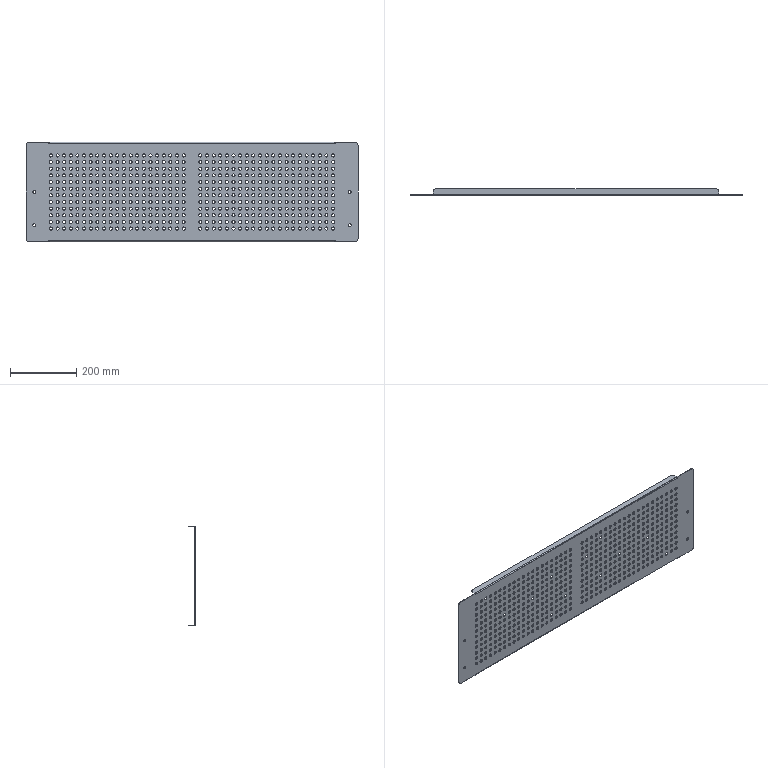Part | SolidWorks | features ICE 2, MirrorPattern 2, EdgeFlange 1, Fillet 1, FlatPattern 1, LPattern 1, SMBaseFlange 1, SheetMetal 1 | 1 solid | 1062 faces | box 1000 x 20 x 300 mm | volume 591466 mm3 | cylinder 1028 | plane 34 | commonest cylinder face diameters 9.2 x1008 9 x8 20 x8 1.473 x2 5.473 x2